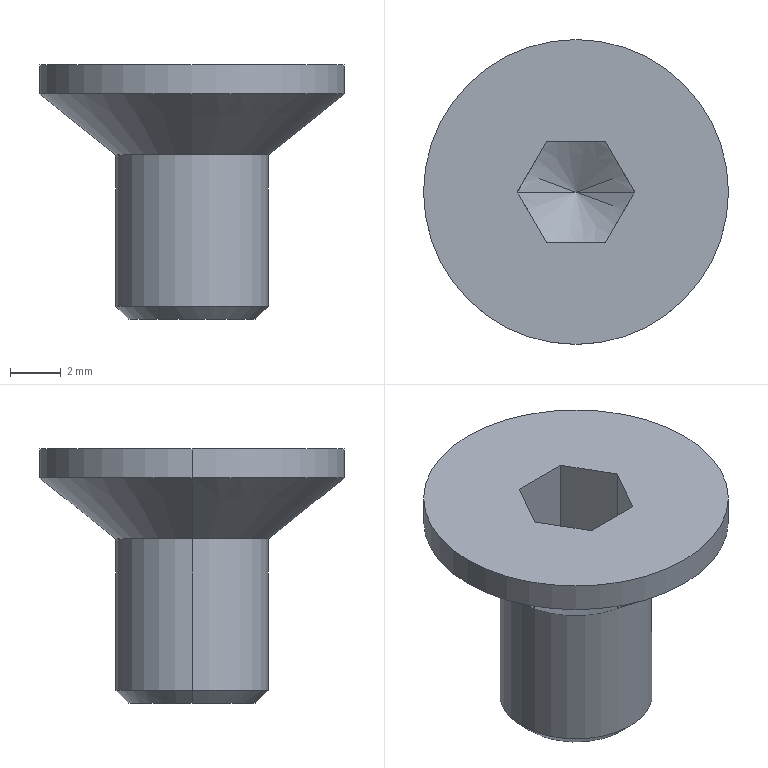Part | Creo | 1 solid | 18 faces | box 12 x 12 x 10 mm | volume 418.882 mm3 | plane 8 | cone 6 | cylinder 4 | commonest cylinder face diameters 6 x2 12 x2
STEP:
#1=CARTESIAN_POINT('',(-327.691,90.995,334.56));
#2=VERTEX_POINT('',#1);
#3=CARTESIAN_POINT('',(-328.845,92.995,334.56));
#4=VERTEX_POINT('',#3);
#5=CARTESIAN_POINT('',(-327.691,90.995,334.56));
#6=CARTESIAN_POINT('',(-327.744,91.088,334.529));
#7=CARTESIAN_POINT('',(-327.852,91.276,334.473));
#8=CARTESIAN_POINT('',(-328.018,91.562,334.412));
#9=CARTESIAN_POINT('',(-328.185,91.851,334.38));
#10=CARTESIAN_POINT('',(-328.352,92.141,334.38));
#11=CARTESIAN_POINT('',(-328.519,92.43,334.412));
#12=CARTESIAN_POINT('',(-328.684,92.716,334.473));
#13=CARTESIAN_POINT('',(-328.792,92.903,334.529));
#14=CARTESIAN_POINT('',(-328.845,92.995,334.56));
#15=B_SPLINE_CURVE_WITH_KNOTS('',3,(#5,#6,#7,#8,#9,#10,#11,#12,#13,#14),.UNSPECIFIED.,.F.,.F.,(4,1,1,1,1,1,1,4),(0.,0.1429,0.2857,0.4286,0.5714,0.7143,0.8571,1.),.UNSPECIFIED.);
#16=EDGE_CURVE('',#2,#4,#15,.T.);
#17=ORIENTED_EDGE('',*,*,#16,.F.);
#18=CARTESIAN_POINT('',(-330.,90.995,333.227));
#19=VERTEX_POINT('',#18);
#20=CARTESIAN_POINT('',(-330.,90.995,333.227));
#21=DIRECTION('',(0.866,0.,0.5));
#22=VECTOR('',#21,2.667);
#23=LINE('',#20,#22);
#24=EDGE_CURVE('',#19,#2,#23,.T.);
#25=ORIENTED_EDGE('',*,*,#24,.F.);
#26=CARTESIAN_POINT('',(-332.309,90.995,334.56));
#27=VERTEX_POINT('',#26);
#28=CARTESIAN_POINT('',(-330.,90.995,333.227));
#29=DIRECTION('',(-0.866,0.,0.5));
#30=VECTOR('',#29,2.667);
#31=LINE('',#28,#30);
#32=EDGE_CURVE('',#19,#27,#31,.T.);
#33=ORIENTED_EDGE('',*,*,#32,.T.);
#34=CARTESIAN_POINT('',(-331.155,92.995,334.56));
#35=VERTEX_POINT('',#34);
#36=CARTESIAN_POINT('',(-331.155,92.995,334.56));
#37=CARTESIAN_POINT('',(-331.208,92.903,334.529));
#38=CARTESIAN_POINT('',(-331.316,92.716,334.473));
#39=CARTESIAN_POINT('',(-331.481,92.43,334.412));
#40=CARTESIAN_POINT('',(-331.648,92.141,334.38));
#41=CARTESIAN_POINT('',(-331.815,91.851,334.38));
#42=CARTESIAN_POINT('',(-331.982,91.562,334.412));
#43=CARTESIAN_POINT('',(-332.148,91.276,334.473));
#44=CARTESIAN_POINT('',(-332.256,91.088,334.529));
#45=CARTESIAN_POINT('',(-332.309,90.995,334.56));
#46=B_SPLINE_CURVE_WITH_KNOTS('',3,(#36,#37,#38,#39,#40,#41,#42,#43,#44,#45),.UNSPECIFIED.,.F.,.F.,(4,1,1,1,1,1,1,4),(0.,0.1429,0.2857,0.4286,0.5714,0.7143,0.8571,1.),.UNSPECIFIED.);
#47=EDGE_CURVE('',#35,#27,#46,.T.);
#48=ORIENTED_EDGE('',*,*,#47,.F.);
#49=CARTESIAN_POINT('',(-328.845,92.995,334.56));
#50=CARTESIAN_POINT('',(-328.903,92.995,334.543));
#51=CARTESIAN_POINT('',(-329.017,92.995,334.512));
#52=CARTESIAN_POINT('',(-329.182,92.995,334.473));
#53=CARTESIAN_POINT('',(-329.344,92.995,334.441));
#54=CARTESIAN_POINT('',(-329.506,92.995,334.415));
#55=CARTESIAN_POINT('',(-329.669,92.995,334.396));
#56=CARTESIAN_POINT('',(-329.834,92.995,334.384));
#57=CARTESIAN_POINT('',(-330.,92.995,334.38));
#58=CARTESIAN_POINT('',(-330.166,92.995,334.384));
#59=CARTESIAN_POINT('',(-330.331,92.995,334.396));
#60=CARTESIAN_POINT('',(-330.494,92.995,334.415));
#61=CARTESIAN_POINT('',(-330.656,92.995,334.441));
#62=CARTESIAN_POINT('',(-330.818,92.995,334.473));
#63=CARTESIAN_POINT('',(-330.983,92.995,334.512));
#64=CARTESIAN_POINT('',(-331.097,92.995,334.543));
#65=CARTESIAN_POINT('',(-331.155,92.995,334.56));
#66=B_SPLINE_CURVE_WITH_KNOTS('',3,(#49,#50,#51,#52,#53,#54,#55,#56,#57,#58,#59,#60,#61,#62,#63,#64,#65),.UNSPECIFIED.,.F.,.F.,(4,1,1,1,1,1,1,1,1,1,1,1,1,1,4),(0.,0.07143,0.1429,0.2143,0.2857,0.3571,0.4286,0.5,0.5714,0.6429,0.7143,0.7857,0.8571,0.9286,1.),.UNSPECIFIED.);
#67=EDGE_CURVE('',#4,#35,#66,.T.);
#68=ORIENTED_EDGE('',*,*,#67,.F.);
#69=EDGE_LOOP('',(#17,#25,#33,#48,#68));
#70=FACE_OUTER_BOUND('',#69,.F.);
#71=CARTESIAN_POINT('',(-330.,90.995,333.907));
#72=DIRECTION('',(0.,0.,1.));
#73=DIRECTION('',(1.,0.,0.));
#74=AXIS2_PLACEMENT_3D('',#71,#72,#73);
#75=CONICAL_SURFACE('',#74,1.178,60.);
#76=ADVANCED_FACE('',(#70),#75,.F.);
#77=CARTESIAN_POINT('',(-328.845,92.995,337.56));
#78=VERTEX_POINT('',#77);
#79=CARTESIAN_POINT('',(-327.691,90.995,337.56));
#80=VERTEX_POINT('',#79);
#81=CARTESIAN_POINT('',(-328.845,92.995,337.56));
#82=DIRECTION('',(0.5,-0.866,0.));
#83=VECTOR('',#82,2.309);
#84=LINE('',#81,#83);
#85=EDGE_CURVE('',#78,#80,#84,.T.);
#86=ORIENTED_EDGE('',*,*,#85,.T.);
#87=CARTESIAN_POINT('',(-327.691,90.995,337.56));
#88=DIRECTION('',(0.,0.,-1.));
#89=VECTOR('',#88,3.);
#90=LINE('',#87,#89);
#91=EDGE_CURVE('',#80,#2,#90,.T.);
#92=ORIENTED_EDGE('',*,*,#91,.T.);
#93=ORIENTED_EDGE('',*,*,#16,.T.);
#94=CARTESIAN_POINT('',(-328.845,92.995,337.56));
#95=DIRECTION('',(0.,0.,-1.));
#96=VECTOR('',#95,3.);
#97=LINE('',#94,#96);
#98=EDGE_CURVE('',#78,#4,#97,.T.);
#99=ORIENTED_EDGE('',*,*,#98,.F.);
#100=EDGE_LOOP('',(#86,#92,#93,#99));
#101=FACE_OUTER_BOUND('',#100,.F.);
#102=CARTESIAN_POINT('',(-327.691,90.995,334.56));
#103=DIRECTION('',(0.866,0.5,0.));
#104=DIRECTION('',(-0.5,0.866,0.));
#105=AXIS2_PLACEMENT_3D('',#102,#103,#104);
#106=PLANE('',#105);
#107=ADVANCED_FACE('',(#101),#106,.F.);
#108=CARTESIAN_POINT('',(-324.,90.995,337.56));
#109=VERTEX_POINT('',#108);
#110=CARTESIAN_POINT('',(-336.,90.995,337.56));
#111=VERTEX_POINT('',#110);
#112=CARTESIAN_POINT('',(-330.,90.995,337.56));
#113=DIRECTION('',(0.,0.,1.));
#114=DIRECTION('',(1.,0.,0.));
#115=AXIS2_PLACEMENT_3D('',#112,#113,#114);
#116=CIRCLE('',#115,6.);
#117=EDGE_CURVE('',#109,#111,#116,.T.);
#118=ORIENTED_EDGE('',*,*,#117,.F.);
#119=CARTESIAN_POINT('',(-330.,90.995,337.56));
#120=DIRECTION('',(0.,0.,1.));
#121=DIRECTION('',(-1.,0.,0.));
#122=AXIS2_PLACEMENT_3D('',#119,#120,#121);
#123=CIRCLE('',#122,6.);
#124=EDGE_CURVE('',#111,#109,#123,.T.);
#125=ORIENTED_EDGE('',*,*,#124,.F.);
#126=EDGE_LOOP('',(#118,#125));
#127=FACE_OUTER_BOUND('',#126,.F.);
#128=CARTESIAN_POINT('',(-331.155,92.995,337.56));
#129=VERTEX_POINT('',#128);
#130=CARTESIAN_POINT('',(-331.155,92.995,337.56));
#131=DIRECTION('',(1.,0.,0.));
#132=VECTOR('',#131,2.309);
#133=LINE('',#130,#132);
#134=EDGE_CURVE('',#129,#78,#133,.T.);
#135=ORIENTED_EDGE('',*,*,#134,.F.);
#136=CARTESIAN_POINT('',(-332.309,90.995,337.56));
#137=VERTEX_POINT('',#136);
#138=CARTESIAN_POINT('',(-332.309,90.995,337.56));
#139=DIRECTION('',(0.5,0.866,0.));
#140=VECTOR('',#139,2.309);
#141=LINE('',#138,#140);
#142=EDGE_CURVE('',#137,#129,#141,.T.);
#143=ORIENTED_EDGE('',*,*,#142,.F.);
#144=CARTESIAN_POINT('',(-331.155,88.995,337.56));
#145=VERTEX_POINT('',#144);
#146=CARTESIAN_POINT('',(-331.155,88.995,337.56));
#147=DIRECTION('',(-0.5,0.866,0.));
#148=VECTOR('',#147,2.309);
#149=LINE('',#146,#148);
#150=EDGE_CURVE('',#145,#137,#149,.T.);
#151=ORIENTED_EDGE('',*,*,#150,.F.);
#152=CARTESIAN_POINT('',(-328.845,88.995,337.56));
#153=VERTEX_POINT('',#152);
#154=CARTESIAN_POINT('',(-328.845,88.995,337.56));
#155=DIRECTION('',(-1.,0.,0.));
#156=VECTOR('',#155,2.309);
#157=LINE('',#154,#156);
#158=EDGE_CURVE('',#153,#145,#157,.T.);
#159=ORIENTED_EDGE('',*,*,#158,.F.);
#160=CARTESIAN_POINT('',(-327.691,90.995,337.56));
#161=DIRECTION('',(-0.5,-0.866,0.));
#162=VECTOR('',#161,2.309);
#163=LINE('',#160,#162);
#164=EDGE_CURVE('',#80,#153,#163,.T.);
#165=ORIENTED_EDGE('',*,*,#164,.F.);
#166=ORIENTED_EDGE('',*,*,#85,.F.);
#167=EDGE_LOOP('',(#135,#143,#151,#159,#165,#166));
#168=FACE_BOUND('',#167,.F.);
#169=CARTESIAN_POINT('',(-324.,90.995,337.56));
#170=DIRECTION('',(0.,0.,-1.));
#171=DIRECTION('',(-1.,0.,0.));
#172=AXIS2_PLACEMENT_3D('',#169,#170,#171);
#173=PLANE('',#172);
#174=ADVANCED_FACE('',(#127,#168),#173,.F.);
#175=ORIENTED_EDGE('',*,*,#134,.T.);
#176=ORIENTED_EDGE('',*,*,#98,.T.);
#177=ORIENTED_EDGE('',*,*,#67,.T.);
#178=CARTESIAN_POINT('',(-331.155,92.995,337.56));
#179=DIRECTION('',(0.,0.,-1.));
#180=VECTOR('',#179,3.);
#181=LINE('',#178,#180);
#182=EDGE_CURVE('',#129,#35,#181,.T.);
#183=ORIENTED_EDGE('',*,*,#182,.F.);
#184=EDGE_LOOP('',(#175,#176,#177,#183));
#185=FACE_OUTER_BOUND('',#184,.F.);
#186=CARTESIAN_POINT('',(-328.845,92.995,334.56));
#187=DIRECTION('',(0.,1.,0.));
#188=DIRECTION('',(0.,0.,1.));
#189=AXIS2_PLACEMENT_3D('',#186,#187,#188);
#190=PLANE('',#189);
#191=ADVANCED_FACE('',(#185),#190,.F.);
#192=ORIENTED_EDGE('',*,*,#142,.T.);
#193=ORIENTED_EDGE('',*,*,#182,.T.);
#194=ORIENTED_EDGE('',*,*,#47,.T.);
#195=CARTESIAN_POINT('',(-332.309,90.995,337.56));
#196=DIRECTION('',(0.,0.,-1.));
#197=VECTOR('',#196,3.);
#198=LINE('',#195,#197);
#199=EDGE_CURVE('',#137,#27,#198,.T.);
#200=ORIENTED_EDGE('',*,*,#199,.F.);
#201=EDGE_LOOP('',(#192,#193,#194,#200));
#202=FACE_OUTER_BOUND('',#201,.F.);
#203=CARTESIAN_POINT('',(-331.155,92.995,334.56));
#204=DIRECTION('',(-0.866,0.5,0.));
#205=DIRECTION('',(-0.5,-0.866,0.));
#206=AXIS2_PLACEMENT_3D('',#203,#204,#205);
#207=PLANE('',#206);
#208=ADVANCED_FACE('',(#202),#207,.F.);
#209=ORIENTED_EDGE('',*,*,#150,.T.);
#210=ORIENTED_EDGE('',*,*,#199,.T.);
#211=CARTESIAN_POINT('',(-331.155,88.995,334.56));
#212=VERTEX_POINT('',#211);
#213=CARTESIAN_POINT('',(-332.309,90.995,334.56));
#214=CARTESIAN_POINT('',(-332.256,90.902,334.529));
#215=CARTESIAN_POINT('',(-332.148,90.715,334.473));
#216=CARTESIAN_POINT('',(-331.982,90.428,334.412));
#217=CARTESIAN_POINT('',(-331.815,90.139,334.38));
#218=CARTESIAN_POINT('',(-331.648,89.85,334.38));
#219=CARTESIAN_POINT('',(-331.481,89.561,334.412));
#220=CARTESIAN_POINT('',(-331.316,89.274,334.473));
#221=CARTESIAN_POINT('',(-331.208,89.088,334.529));
#222=CARTESIAN_POINT('',(-331.155,88.995,334.56));
#223=B_SPLINE_CURVE_WITH_KNOTS('',3,(#213,#214,#215,#216,#217,#218,#219,#220,#221,#222),.UNSPECIFIED.,.F.,.F.,(4,1,1,1,1,1,1,4),(0.,0.1429,0.2857,0.4286,0.5714,0.7143,0.8571,1.),.UNSPECIFIED.);
#224=EDGE_CURVE('',#27,#212,#223,.T.);
#225=ORIENTED_EDGE('',*,*,#224,.T.);
#226=CARTESIAN_POINT('',(-331.155,88.995,337.56));
#227=DIRECTION('',(0.,0.,-1.));
#228=VECTOR('',#227,3.);
#229=LINE('',#226,#228);
#230=EDGE_CURVE('',#145,#212,#229,.T.);
#231=ORIENTED_EDGE('',*,*,#230,.F.);
#232=EDGE_LOOP('',(#209,#210,#225,#231));
#233=FACE_OUTER_BOUND('',#232,.F.);
#234=CARTESIAN_POINT('',(-332.309,90.995,334.56));
#235=DIRECTION('',(-0.866,-0.5,0.));
#236=DIRECTION('',(0.5,-0.866,0.));
#237=AXIS2_PLACEMENT_3D('',#234,#235,#236);
#238=PLANE('',#237);
#239=ADVANCED_FACE('',(#233),#238,.F.);
#240=CARTESIAN_POINT('',(-328.845,88.995,334.56));
#241=VERTEX_POINT('',#240);
#242=CARTESIAN_POINT('',(-331.155,88.995,334.56));
#243=CARTESIAN_POINT('',(-331.097,88.995,334.543));
#244=CARTESIAN_POINT('',(-330.983,88.995,334.512));
#245=CARTESIAN_POINT('',(-330.818,88.995,334.473));
#246=CARTESIAN_POINT('',(-330.656,88.995,334.441));
#247=CARTESIAN_POINT('',(-330.494,88.995,334.415));
#248=CARTESIAN_POINT('',(-330.331,88.995,334.396));
#249=CARTESIAN_POINT('',(-330.166,88.995,334.384));
#250=CARTESIAN_POINT('',(-330.,88.995,334.38));
#251=CARTESIAN_POINT('',(-329.834,88.995,334.384));
#252=CARTESIAN_POINT('',(-329.669,88.995,334.396));
#253=CARTESIAN_POINT('',(-329.506,88.995,334.415));
#254=CARTESIAN_POINT('',(-329.344,88.995,334.441));
#255=CARTESIAN_POINT('',(-329.182,88.995,334.473));
#256=CARTESIAN_POINT('',(-329.017,88.995,334.512));
#257=CARTESIAN_POINT('',(-328.903,88.995,334.543));
#258=CARTESIAN_POINT('',(-328.845,88.995,334.56));
#259=B_SPLINE_CURVE_WITH_KNOTS('',3,(#242,#243,#244,#245,#246,#247,#248,#249,#250,#251,#252,#253,#254,#255,#256,#257,#258),.UNSPECIFIED.,.F.,.F.,(4,1,1,1,1,1,1,1,1,1,1,1,1,1,4),(0.,0.07143,0.1429,0.2143,0.2857,0.3571,0.4286,0.5,0.5714,0.6429,0.7143,0.7857,0.8571,0.9286,1.),.UNSPECIFIED.);
#260=EDGE_CURVE('',#212,#241,#259,.T.);
#261=ORIENTED_EDGE('',*,*,#260,.F.);
#262=ORIENTED_EDGE('',*,*,#224,.F.);
#263=ORIENTED_EDGE('',*,*,#32,.F.);
#264=ORIENTED_EDGE('',*,*,#24,.T.);
#265=CARTESIAN_POINT('',(-328.845,88.995,334.56));
#266=CARTESIAN_POINT('',(-328.792,89.088,334.529));
#267=CARTESIAN_POINT('',(-328.684,89.274,334.473));
#268=CARTESIAN_POINT('',(-328.519,89.561,334.412));
#269=CARTESIAN_POINT('',(-328.352,89.85,334.38));
#270=CARTESIAN_POINT('',(-328.185,90.139,334.38));
#271=CARTESIAN_POINT('',(-328.018,90.428,334.412));
#272=CARTESIAN_POINT('',(-327.852,90.715,334.473));
#273=CARTESIAN_POINT('',(-327.744,90.902,334.529));
#274=CARTESIAN_POINT('',(-327.691,90.995,334.56));
#275=B_SPLINE_CURVE_WITH_KNOTS('',3,(#265,#266,#267,#268,#269,#270,#271,#272,#273,#274),.UNSPECIFIED.,.F.,.F.,(4,1,1,1,1,1,1,4),(0.,0.1429,0.2857,0.4286,0.5714,0.7143,0.8571,1.),.UNSPECIFIED.);
#276=EDGE_CURVE('',#241,#2,#275,.T.);
#277=ORIENTED_EDGE('',*,*,#276,.F.);
#278=EDGE_LOOP('',(#261,#262,#263,#264,#277));
#279=FACE_OUTER_BOUND('',#278,.F.);
#280=CARTESIAN_POINT('',(-330.,90.995,333.907));
#281=DIRECTION('',(0.,0.,1.));
#282=DIRECTION('',(1.,0.,0.));
#283=AXIS2_PLACEMENT_3D('',#280,#281,#282);
#284=CONICAL_SURFACE('',#283,1.178,60.);
#285=ADVANCED_FACE('',(#279),#284,.F.);
#286=ORIENTED_EDGE('',*,*,#158,.T.);
#287=ORIENTED_EDGE('',*,*,#230,.T.);
#288=ORIENTED_EDGE('',*,*,#260,.T.);
#289=CARTESIAN_POINT('',(-328.845,88.995,337.56));
#290=DIRECTION('',(0.,0.,-1.));
#291=VECTOR('',#290,3.);
#292=LINE('',#289,#291);
#293=EDGE_CURVE('',#153,#241,#292,.T.);
#294=ORIENTED_EDGE('',*,*,#293,.F.);
#295=EDGE_LOOP('',(#286,#287,#288,#294));
#296=FACE_OUTER_BOUND('',#295,.F.);
#297=CARTESIAN_POINT('',(-331.155,88.995,334.56));
#298=DIRECTION('',(0.,-1.,0.));
#299=DIRECTION('',(0.,0.,-1.));
#300=AXIS2_PLACEMENT_3D('',#297,#298,#299);
#301=PLANE('',#300);
#302=ADVANCED_FACE('',(#296),#301,.F.);
#303=ORIENTED_EDGE('',*,*,#164,.T.);
#304=ORIENTED_EDGE('',*,*,#293,.T.);
#305=ORIENTED_EDGE('',*,*,#276,.T.);
#306=ORIENTED_EDGE('',*,*,#91,.F.);
#307=EDGE_LOOP('',(#303,#304,#305,#306));
#308=FACE_OUTER_BOUND('',#307,.F.);
#309=CARTESIAN_POINT('',(-328.845,88.995,334.56));
#310=DIRECTION('',(0.866,-0.5,0.));
#311=DIRECTION('',(0.5,0.866,0.));
#312=AXIS2_PLACEMENT_3D('',#309,#310,#311);
#313=PLANE('',#312);
#314=ADVANCED_FACE('',(#308),#313,.F.);
#315=ORIENTED_EDGE('',*,*,#117,.T.);
#316=CARTESIAN_POINT('',(-336.,90.995,336.42));
#317=VERTEX_POINT('',#316);
#318=CARTESIAN_POINT('',(-336.,90.995,336.42));
#319=DIRECTION('',(0.,0.,1.));
#320=VECTOR('',#319,1.14);
#321=LINE('',#318,#320);
#322=EDGE_CURVE('',#317,#111,#321,.T.);
#323=ORIENTED_EDGE('',*,*,#322,.F.);
#324=CARTESIAN_POINT('',(-324.,90.995,336.42));
#325=VERTEX_POINT('',#324);
#326=CARTESIAN_POINT('',(-330.,90.995,336.42));
#327=DIRECTION('',(0.,0.,-1.));
#328=DIRECTION('',(-1.,0.,0.));
#329=AXIS2_PLACEMENT_3D('',#326,#327,#328);
#330=CIRCLE('',#329,6.);
#331=EDGE_CURVE('',#317,#325,#330,.T.);
#332=ORIENTED_EDGE('',*,*,#331,.T.);
#333=CARTESIAN_POINT('',(-324.,90.995,336.42));
#334=DIRECTION('',(0.,0.,1.));
#335=VECTOR('',#334,1.14);
#336=LINE('',#333,#335);
#337=EDGE_CURVE('',#325,#109,#336,.T.);
#338=ORIENTED_EDGE('',*,*,#337,.T.);
#339=EDGE_LOOP('',(#315,#323,#332,#338));
#340=FACE_OUTER_BOUND('',#339,.F.);
#341=CARTESIAN_POINT('',(-330.,90.995,338.56));
#342=DIRECTION('',(0.,0.,1.));
#343=DIRECTION('',(1.,0.,0.));
#344=AXIS2_PLACEMENT_3D('',#341,#342,#343);
#345=CYLINDRICAL_SURFACE('',#344,6.);
#346=ADVANCED_FACE('',(#340),#345,.T.);
#347=ORIENTED_EDGE('',*,*,#124,.T.);
#348=ORIENTED_EDGE('',*,*,#337,.F.);
#349=CARTESIAN_POINT('',(-330.,90.995,336.42));
#350=DIRECTION('',(0.,0.,-1.));
#351=DIRECTION('',(1.,0.,0.));
#352=AXIS2_PLACEMENT_3D('',#349,#350,#351);
#353=CIRCLE('',#352,6.);
#354=EDGE_CURVE('',#325,#317,#353,.T.);
#355=ORIENTED_EDGE('',*,*,#354,.T.);
#356=ORIENTED_EDGE('',*,*,#322,.T.);
#357=EDGE_LOOP('',(#347,#348,#355,#356));
#358=FACE_OUTER_BOUND('',#357,.F.);
#359=CARTESIAN_POINT('',(-330.,90.995,338.56));
#360=DIRECTION('',(0.,0.,1.));
#361=DIRECTION('',(1.,0.,0.));
#362=AXIS2_PLACEMENT_3D('',#359,#360,#361);
#363=CYLINDRICAL_SURFACE('',#362,6.);
#364=ADVANCED_FACE('',(#358),#363,.T.);
#365=CARTESIAN_POINT('',(-333.,90.995,334.02));
#366=VERTEX_POINT('',#365);
#367=CARTESIAN_POINT('',(-327.,90.995,334.02));
#368=VERTEX_POINT('',#367);
#369=CARTESIAN_POINT('',(-330.,90.995,334.02));
#370=DIRECTION('',(0.,0.,1.));
#371=DIRECTION('',(-1.,0.,0.));
#372=AXIS2_PLACEMENT_3D('',#369,#370,#371);
#373=CIRCLE('',#372,3.);
#374=EDGE_CURVE('',#366,#368,#373,.T.);
#375=ORIENTED_EDGE('',*,*,#374,.F.);
#376=CARTESIAN_POINT('',(-333.,90.995,334.02));
#377=DIRECTION('',(-0.7809,0.,0.6247));
#378=VECTOR('',#377,3.842);
#379=LINE('',#376,#378);
#380=EDGE_CURVE('',#366,#317,#379,.T.);
#381=ORIENTED_EDGE('',*,*,#380,.T.);
#382=ORIENTED_EDGE('',*,*,#354,.F.);
#383=CARTESIAN_POINT('',(-327.,90.995,334.02));
#384=DIRECTION('',(0.7809,0.,0.6247));
#385=VECTOR('',#384,3.842);
#386=LINE('',#383,#385);
#387=EDGE_CURVE('',#368,#325,#386,.T.);
#388=ORIENTED_EDGE('',*,*,#387,.F.);
#389=EDGE_LOOP('',(#375,#381,#382,#388));
#390=FACE_OUTER_BOUND('',#389,.F.);
#391=CARTESIAN_POINT('',(-330.,90.995,335.22));
#392=DIRECTION('',(0.,0.,1.));
#393=DIRECTION('',(1.,0.,0.));
#394=AXIS2_PLACEMENT_3D('',#391,#392,#393);
#395=CONICAL_SURFACE('',#394,4.5,51.34);
#396=ADVANCED_FACE('',(#390),#395,.T.);
#397=ORIENTED_EDGE('',*,*,#374,.T.);
#398=CARTESIAN_POINT('',(-327.,90.995,328.06));
#399=VERTEX_POINT('',#398);
#400=CARTESIAN_POINT('',(-327.,90.995,328.06));
#401=DIRECTION('',(0.,0.,1.));
#402=VECTOR('',#401,5.96);
#403=LINE('',#400,#402);
#404=EDGE_CURVE('',#399,#368,#403,.T.);
#405=ORIENTED_EDGE('',*,*,#404,.F.);
#406=CARTESIAN_POINT('',(-333.,90.995,328.06));
#407=VERTEX_POINT('',#406);
#408=CARTESIAN_POINT('',(-330.,90.995,328.06));
#409=DIRECTION('',(0.,0.,-1.));
#410=DIRECTION('',(1.,0.,0.));
#411=AXIS2_PLACEMENT_3D('',#408,#409,#410);
#412=CIRCLE('',#411,3.);
#413=EDGE_CURVE('',#399,#407,#412,.T.);
#414=ORIENTED_EDGE('',*,*,#413,.T.);
#415=CARTESIAN_POINT('',(-333.,90.995,328.06));
#416=DIRECTION('',(0.,0.,1.));
#417=VECTOR('',#416,5.96);
#418=LINE('',#415,#417);
#419=EDGE_CURVE('',#407,#366,#418,.T.);
#420=ORIENTED_EDGE('',*,*,#419,.T.);
#421=EDGE_LOOP('',(#397,#405,#414,#420));
#422=FACE_OUTER_BOUND('',#421,.F.);
#423=CARTESIAN_POINT('',(-330.,90.995,338.56));
#424=DIRECTION('',(0.,0.,1.));
#425=DIRECTION('',(1.,0.,0.));
#426=AXIS2_PLACEMENT_3D('',#423,#424,#425);
#427=CYLINDRICAL_SURFACE('',#426,3.);
#428=ADVANCED_FACE('',(#422),#427,.T.);
#429=CARTESIAN_POINT('',(-330.,90.995,334.02));
#430=DIRECTION('',(0.,0.,1.));
#431=DIRECTION('',(1.,0.,0.));
#432=AXIS2_PLACEMENT_3D('',#429,#430,#431);
#433=CIRCLE('',#432,3.);
#434=EDGE_CURVE('',#368,#366,#433,.T.);
#435=ORIENTED_EDGE('',*,*,#434,.T.);
#436=ORIENTED_EDGE('',*,*,#419,.F.);
#437=CARTESIAN_POINT('',(-330.,90.995,328.06));
#438=DIRECTION('',(0.,0.,-1.));
#439=DIRECTION('',(-1.,0.,0.));
#440=AXIS2_PLACEMENT_3D('',#437,#438,#439);
#441=CIRCLE('',#440,3.);
#442=EDGE_CURVE('',#407,#399,#441,.T.);
#443=ORIENTED_EDGE('',*,*,#442,.T.);
#444=ORIENTED_EDGE('',*,*,#404,.T.);
#445=EDGE_LOOP('',(#435,#436,#443,#444));
#446=FACE_OUTER_BOUND('',#445,.F.);
#447=CARTESIAN_POINT('',(-330.,90.995,338.56));
#448=DIRECTION('',(0.,0.,1.));
#449=DIRECTION('',(1.,0.,0.));
#450=AXIS2_PLACEMENT_3D('',#447,#448,#449);
#451=CYLINDRICAL_SURFACE('',#450,3.);
#452=ADVANCED_FACE('',(#446),#451,.T.);
#453=ORIENTED_EDGE('',*,*,#434,.F.);
#454=ORIENTED_EDGE('',*,*,#387,.T.);
#455=ORIENTED_EDGE('',*,*,#331,.F.);
#456=ORIENTED_EDGE('',*,*,#380,.F.);
#457=EDGE_LOOP('',(#453,#454,#455,#456));
#458=FACE_OUTER_BOUND('',#457,.F.);
#459=CARTESIAN_POINT('',(-330.,90.995,335.22));
#460=DIRECTION('',(0.,0.,1.));
#461=DIRECTION('',(1.,0.,0.));
#462=AXIS2_PLACEMENT_3D('',#459,#460,#461);
#463=CONICAL_SURFACE('',#462,4.5,51.34);
#464=ADVANCED_FACE('',(#458),#463,.T.);
#465=ORIENTED_EDGE('',*,*,#442,.F.);
#466=CARTESIAN_POINT('',(-332.5,90.995,327.56));
#467=VERTEX_POINT('',#466);
#468=CARTESIAN_POINT('',(-332.5,90.995,327.56));
#469=DIRECTION('',(-0.7071,0.,0.7071));
#470=VECTOR('',#469,0.7071);
#471=LINE('',#468,#470);
#472=EDGE_CURVE('',#467,#407,#471,.T.);
#473=ORIENTED_EDGE('',*,*,#472,.F.);
#474=CARTESIAN_POINT('',(-327.5,90.995,327.56));
#475=VERTEX_POINT('',#474);
#476=CARTESIAN_POINT('',(-330.,90.995,327.56));
#477=DIRECTION('',(0.,0.,-1.));
#478=DIRECTION('',(-1.,0.,0.));
#479=AXIS2_PLACEMENT_3D('',#476,#477,#478);
#480=CIRCLE('',#479,2.5);
#481=EDGE_CURVE('',#467,#475,#480,.T.);
#482=ORIENTED_EDGE('',*,*,#481,.T.);
#483=CARTESIAN_POINT('',(-327.5,90.995,327.56));
#484=DIRECTION('',(0.7071,0.,0.7071));
#485=VECTOR('',#484,0.7071);
#486=LINE('',#483,#485);
#487=EDGE_CURVE('',#475,#399,#486,.T.);
#488=ORIENTED_EDGE('',*,*,#487,.T.);
#489=EDGE_LOOP('',(#465,#473,#482,#488));
#490=FACE_OUTER_BOUND('',#489,.F.);
#491=CARTESIAN_POINT('',(-330.,90.995,327.81));
#492=DIRECTION('',(0.,0.,1.));
#493=DIRECTION('',(1.,0.,0.));
#494=AXIS2_PLACEMENT_3D('',#491,#492,#493);
#495=CONICAL_SURFACE('',#494,2.75,45.);
#496=ADVANCED_FACE('',(#490),#495,.T.);
#497=ORIENTED_EDGE('',*,*,#413,.F.);
#498=ORIENTED_EDGE('',*,*,#487,.F.);
#499=CARTESIAN_POINT('',(-330.,90.995,327.56));
#500=DIRECTION('',(0.,0.,-1.));
#501=DIRECTION('',(1.,0.,0.));
#502=AXIS2_PLACEMENT_3D('',#499,#500,#501);
#503=CIRCLE('',#502,2.5);
#504=EDGE_CURVE('',#475,#467,#503,.T.);
#505=ORIENTED_EDGE('',*,*,#504,.T.);
#506=ORIENTED_EDGE('',*,*,#472,.T.);
#507=EDGE_LOOP('',(#497,#498,#505,#506));
#508=FACE_OUTER_BOUND('',#507,.F.);
#509=CARTESIAN_POINT('',(-330.,90.995,327.81));
#510=DIRECTION('',(0.,0.,1.));
#511=DIRECTION('',(1.,0.,0.));
#512=AXIS2_PLACEMENT_3D('',#509,#510,#511);
#513=CONICAL_SURFACE('',#512,2.75,45.);
#514=ADVANCED_FACE('',(#508),#513,.T.);
#515=ORIENTED_EDGE('',*,*,#504,.F.);
#516=ORIENTED_EDGE('',*,*,#481,.F.);
#517=EDGE_LOOP('',(#515,#516));
#518=FACE_OUTER_BOUND('',#517,.F.);
#519=CARTESIAN_POINT('',(-330.,90.995,327.56));
#520=DIRECTION('',(0.,0.,1.));
#521=DIRECTION('',(1.,0.,0.));
#522=AXIS2_PLACEMENT_3D('',#519,#520,#521);
#523=PLANE('',#522);
#524=ADVANCED_FACE('',(#518),#523,.F.);
#525=CLOSED_SHELL('',(#76,#107,#174,#191,#208,#239,#285,#302,#314,#346,#364,#396,#428,#452,#464,#496,#514,#524));
#526=MANIFOLD_SOLID_BREP('',#525);
#527=(LENGTH_UNIT()NAMED_UNIT(*)SI_UNIT(.MILLI.,.METRE.));
#528=UNCERTAINTY_MEASURE_WITH_UNIT(LENGTH_MEASURE(0.00197),#527,'','');
#529=(NAMED_UNIT(*)PLANE_ANGLE_UNIT()SI_UNIT($,.RADIAN.));
#530=PLANE_ANGLE_MEASURE_WITH_UNIT(PLANE_ANGLE_MEASURE(0.01745),#529);
#531=(CONVERSION_BASED_UNIT('DEGREE',#530)NAMED_UNIT(*)PLANE_ANGLE_UNIT());
#532=(NAMED_UNIT(*)SI_UNIT($,.STERADIAN.)SOLID_ANGLE_UNIT());
#533=(GEOMETRIC_REPRESENTATION_CONTEXT(3)GLOBAL_UNCERTAINTY_ASSIGNED_CONTEXT((#528))GLOBAL_UNIT_ASSIGNED_CONTEXT((#527,#531,#532))REPRESENTATION_CONTEXT('',''));
#534=ADVANCED_BREP_SHAPE_REPRESENTATION('',(#526),#533);